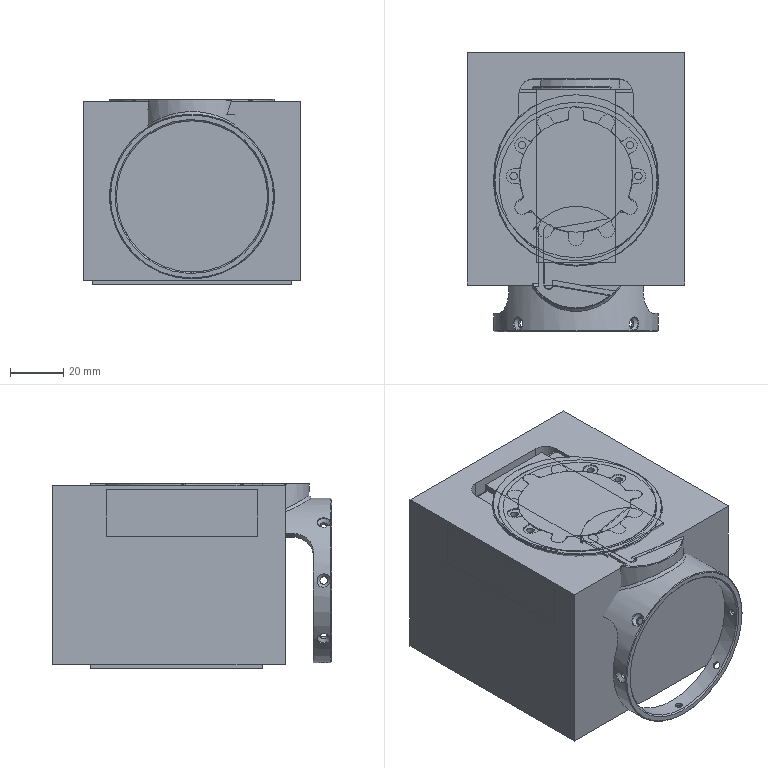NC program | NX | posted with a generic post | part box 82 x 105.2 x 70 mm
Whole program:
N10 G17 G21 G94 G90
(外形动态铣_1 , TOOL : 粗刀D16)
N12 T18 M6
N14 G53
N16 G17 G0 G90 X-3.784 Y5.106 B0. C0. S5500 M3
N18 G43 Z11. H18
N20 G94 G1 Z1. F3500.
N22 G3 X-3.784 Y5.106 Z-0.404 I3.765 J-5.175
N24 X-3.784 Y5.106 Z-1.808 I3.765 J-5.175
N26 X-3.784 Y5.106 Z-3.213 I3.765 J-5.175
N28 X-3.784 Y5.106 Z-4.617 I3.765 J-5.175
N30 X-3.784 Y5.106 Z-6.021 I3.765 J-5.175
N32 X-3.784 Y5.106 Z-7.425 I3.765 J-5.175
N34 X-3.784 Y5.106 Z-8.83 I3.765 J-5.175
N36 X-3.784 Y5.106 Z-10.234 I3.765 J-5.175
N38 X-3.784 Y5.106 Z-11.638 I3.765 J-5.175
N40 X-3.784 Y5.106 Z-13.042 I3.765 J-5.175
N42 X-3.784 Y5.106 Z-14.447 I3.765 J-5.175
N44 X-3.784 Y5.106 Z-15.851 I3.765 J-5.175
N46 X-3.784 Y5.106 Z-17.255 I3.765 J-5.175
N48 X-3.784 Y5.106 Z-18.659 I3.765 J-5.175
N50 X-3.784 Y5.106 Z-20.064 I3.765 J-5.175
N52 X-3.784 Y5.106 Z-21.468 I3.765 J-5.175
N54 X-3.784 Y5.106 Z-22.872 I3.765 J-5.175
N56 X-3.784 Y5.106 Z-24.276 I3.765 J-5.175
N58 X-3.784 Y5.106 Z-25.681 I3.765 J-5.175
N60 X-3.784 Y5.106 Z-27.085 I3.765 J-5.175
N62 X6.381 Y0.001 Z-28. R-6.4
N64 X-6.159 Y-1.924 R-6.417
N66 X5.583 Y-3.213 R6.447
N68 X4.619 Y5.05 R6.617
N70 X-2.015 Y6.615 R6.783
N72 X-1.429 Y-6.792 R6.922
N74 X5.428 Y-4.327 R6.966
N76 X5.458 Y4.871 R7.189
N78 X-1.347 Y7.296 R7.232
N80 X-3.143 Y-6.759 R7.43
N82 X5.315 Y-5.233 R7.495
N84 X6.334 Y4.554 R7.735
N86 X-1.413 Y7.816 R7.718
N88 X-3.194 Y-7.315 R7.955
N90 X5.195 Y-6.068 R8.031
N92 X7.227 Y4.092 R8.265
N94 X-0.67 Y8.452 R8.235
N96 X-7.198 Y-4.572 R8.485
N98 X4.491 Y-7.254 R8.542
N100 X7.344 Y4.986 R8.811
N102 X-2.79 Y8.608 R8.838
N104 X0.22 Y-9.083 R9.064
N106 X8.483 Y-3.519 R9.312
N108 X0.238 Y9.593 R9.335
N110 X-9.345 Y-2.455 R9.605
N112 X3.895 Y-8.848 R9.664
N114 X-0.068 Y10.184 R9.927
N116 X-10.127 Y-1.586 R10.185
N118 X3.436 Y-9.665 R10.249
N120 X0.291 Y10.777 R10.523
N122 X-10.229 Y-3.64 R10.794
N124 X3.073 Y-10.423 R10.868
N126 X0.292 Y11.389 R11.134
N128 X-11.409 Y-1.191 R11.396
N130 X3.05 Y-11.073 R11.48
N132 X0.983 Y11.971 R11.754
N134 X-12.028 Y1.278 R12.002
N136 X2.128 Y-11.927 R12.101
N138 X10.461 Y6.804 R12.376
N140 X-3.616 Y12.16 R12.464
N142 X-12.426 Y-2.837 R12.684
N144 X3.778 Y-12.193 R12.774
N146 X7.36 Y10.98 R13.028
N148 X-7.611 Y10.983 R13.201
N150 X-9.364 Y-9.587 R13.365
N152 X7.293 Y-11.291 R13.474
N154 X9.935 Y9.622 R13.683
N156 X-5.912 Y12.705 R13.82
N158 X-10.732 Y-9.093 R14.017
N160 X5.879 Y-12.813 R14.13
N162 X12.17 Y7.794 R14.342
N164 X-4.674 Y13.912 R14.454
N166 X-13.994 Y-4.617 R14.665
N168 X3.837 Y-14.256 R14.772
N170 X13.816 Y6.068 R15.006
N172 X-3.359 Y14.976 R15.109
N174 X-15.363 Y-1.292 R15.338
N176 X0.655 Y-15.424 R15.44
N178 X14.873 Y-4.712 R15.662
N180 X1.02 Y15.975 R15.77
N182 X-15.835 Y2.94 R15.998
N184 X-2.629 Y-15.909 R16.112
N186 X14.797 Y-6.767 R16.314
N188 X5.904 Y15.577 R16.449
N190 X-12.186 Y11.541 R16.613
N192 X-4.873 Y-16.102 R16.788
N194 X14.677 Y-8.494 R16.994
N196 X6.511 Y16.093 R17.151
N198 X-11.938 Y12.781 R17.303
N200 X-10.446 Y-14.08 R17.485
N202 X14.162 Y-10.535 R17.678
N204 X6.516 Y16.862 R17.862
N206 X-10.879 Y14.594 R18.008
N208 X-6.335 Y-17.116 R18.211
N210 X15.82 Y-9.382 R18.411
N212 X7.383 Y17.28 R18.587
N214 X-10.698 Y15.613 R18.722
N216 X-7.508 Y-17.431 R18.939
N218 X16.802 Y-9.147 R19.139
N220 X8.107 Y17.755 R19.32
N222 X-14.492 Y13.299 R19.465
N224 X-7.242 Y-18.336 R19.676
N226 X16.749 Y-10.661 R19.864
N228 X7.622 Y18.773 R20.055
N230 X-14.319 Y14.538 R20.185
N232 X-7.55 Y-19.009 R20.409
N234 X17.983 Y-10.066 R20.598
N236 X9.019 Y18.959 R20.799
N238 X-13.831 Y16.001 R20.934
N240 X-9.758 Y-18.822 R21.158
N242 X17.341 Y-12.438 R21.333
N244 X8.342 Y20.092 R21.557
N246 X-14.15 Y16.715 R21.672
N248 X-21.896 Y1.274 R21.879
N250 X-9.379 Y-19.854 R21.91
N252 X9.291 Y-19.973 R22.044
N254 X21.998 Y3.456 R22.247
N256 X5.042 Y21.975 R22.363
N258 X-12.269 Y19.039 R22.33
N260 X-22.588 Y2.165 R22.602
N262 X-18.471 Y-13.214 R22.645
N264 X4.912 Y-22.232 R22.818
N266 X10.783 Y-20.084 R23.104
N268 X16.696 Y15.519 R22.794
N270 G2 X15.722 Y16.62 R18.325
N272 G3 X12.958 Y19.176 R15.261
N274 X5.207 Y22.713 R21.966
N276 X-14.081 Y18.713 R23.157
N278 G1 X-14.407 Y18.466
N280 G3 X-14.7 Y18.163 R1.237
N282 G2 X-16.194 Y16.064 R10.91
N284 G3 X-18.085 Y13.88 R29.531
N286 X10.872 Y-20.036 R22.796
N288 X11.323 Y-19.376 R0.88
N290 G1 X11.502 Y-17.996
N292 X11.861 Y-15.219 Z-27.5
N294 X15.344 Y11.699 F15000.
N296 X15.704 Y14.476 Z-28. F3500.
N298 X15.897 Y15.97
N300 G3 X15.722 Y16.62 R0.88
N302 G2 X14.962 Y17.705 R13.92
N304 G3 X13.465 Y19.422 R8.461
N306 X9.979 Y21.752 R16.288
N308 X1.125 Y24.078 R22.494
N310 X-13.106 Y20.318 R23.892
N312 X-13.908 Y19.712 R6.441
N314 X-14.119 Y19.384 R1.156
N316 G2 X-14.721 Y18.126 R9.352
N318 G3 X-14.119 Y19.384 R9.352
N320 G1 X-14.029 Y19.617
N322 G2 X-13.258 Y20.558 R4.444
N324 X-11.121 Y22.12 R11.56
N326 X-6.152 Y24.122 R20.064
N328 X8.694 Y23.164 R23.732
N330 X13.001 Y20.706 R18.073
N332 X13.798 Y20.014 R10.677
N334 X14.001 Y19.687 R1.168
N336 G3 X14.962 Y17.705 R11.57
N338 G2 X14.001 Y19.687 R11.57
N340 G1 X13.933 Y19.864
N342 X13.928 Y19.878
N344 G3 X13.549 Y20.508 R2.958
N346 X11.795 Y22.164 R8.411
N348 X8.327 Y24.05 R16.01
N350 X0.534 Y25.637 R22.912
N352 X-8.61 Y24.13 R23.643
N354 X-11.988 Y22.402 R16.692
N356 X-13.452 Y21.178 R8.868
N358 X-13.647 Y20.823 R1.259
N360 G2 X-14.07 Y19.51 R9.633
N362 G3 X-13.647 Y20.823 R9.633
N364 G1 X-13.614 Y20.945
N366 X-13.608 Y20.97
N368 G2 X-13.432 Y21.357 R1.713
N370 X-12.263 Y22.691 R5.793
N372 X-9.129 Y24.615 R13.04
N374 X-3.244 Y26.219 R21.115
N376 X7.354 Y25.21 R23.909
N378 X11.351 Y23.303 R17.579
N380 X13.349 Y21.618 R9.929
N382 X13.553 Y21.23 R1.212
N384 G3 X13.928 Y19.878 R10.647
N386 G2 X13.553 Y21.23 R10.647
N388 G1 X13.527 Y21.353
N390 X13.496 Y21.474
N392 G3 X12.861 Y22.498 R4.095
N394 X11.022 Y24.122 R9.022
N396 X7.193 Y25.992 R15.979
N398 X-0.669 Y27.179 R23.165
N400 X-7.952 Y25.882 R22.825
N402 X-11.398 Y24.162 R15.64
N404 X-13.21 Y22.518 R8.421
N406 X-13.406 Y22.05 R1.101
N408 G2 X-13.608 Y20.97 R12.038
N410 G3 X-13.406 Y22.05 R12.038
N412 G1 X-13.377 Y22.302
N414 G2 X-12.763 Y23.399 R3.705
N416 X-11.222 Y24.846 R7.832
N418 X-7.996 Y26.564 R13.855
N420 X-3.514 Y27.704 R20.945
N422 X5.203 Y27.341 R23.775
N424 X9.416 Y25.86 R19.684
N426 X12.132 Y24.078 R12.486
N428 X13.222 Y22.868 R6.56
N430 X13.353 Y22.492 R1.266
N432 G3 X13.55 Y21.246 R10.987
N434 G2 X13.353 Y22.492 R10.987
N436 G1 X13.345 Y22.581
N438 X13.344 Y22.593
N440 X13.334 Y22.717
N442 G3 X12.779 Y23.815 R3.526
N444 X11.481 Y25.166 R7.411
N446 X8.291 Y27.063 R13.05
N448 X2.962 Y28.5 R20.694
N450 G1 X-2.038
N452 G3 X-8.998 Y26.91 R18.276
N454 X-11.775 Y25.212 R12.397
N456 X-13.142 Y23.717 R6.721
N458 X-13.31 Y23.214 R1.078
N460 G2 X-13.389 Y22.203 R8.714
N462 G3 X-13.31 Y23.214 R8.714
N464 G1 X-13.305 Y23.464
N466 G2 X-12.793 Y24.583 R3.38
N468 X-11.299 Y26.149 R7.293
N470 X-8.123 Y27.957 R12.789
N472 X-6.711 Y28.455 R16.875
N474 X-6.441 Y28.5 R1.43
N476 G1 X-1.941
N478 X-7.066
N480 G3 X-9.313 Y27.948 R7.391
N482 X-12.162 Y26.111 R9.158
N484 X-13.166 Y24.839 R5.937
N486 X-13.3 Y24.344 R1.098
N488 G1 Y23.678
N490 X-13.306 Y23.419
N492 X-13.3 Y23.669
N494 Y23.678
N496 Y24.594
N498 G2 X-12.833 Y25.744 R3.222
N500 X-10.942 Y27.638 R6.743
N502 X-9.454 Y28.442 R8.231
N504 X-9.164 Y28.5 R1.394
N506 G1 X-7.039
N508 X-9.414
N510 G3 X-10.929 Y28.029 R4.247
N512 X-13.19 Y25.899 R5.46
N514 X-13.3 Y25.489 R1.231
N516 G1 Y24.489
N518 Y25.614
N520 X-13.296 Y25.739
N522 G2 X-12.781 Y26.887 R3.143
N524 X-10.991 Y28.414 R4.876
N526 X-10.604 Y28.5 R1.271
N528 G1 X-9.354
N530 X-10.854
N532 G3 X-12.043 Y28.014 R3.036
N534 X-13.197 Y26.781 R3.655
N536 X-13.3 Y26.379 R1.245
N538 G1 Y25.504
N540 Y26.504
N542 X-13.297 Y26.629
N544 G2 X-12.908 Y27.489 R2.417
N546 X-11.914 Y28.39 R3.041
N548 X-11.504 Y28.5 R1.231
N550 G1 X-10.754
N552 X-11.629
N554 X-11.754 Y28.495
N556 G3 X-12.344 Y28.261 R2.142
N558 X-13.14 Y27.51 R2.729
N560 X-13.3 Y27.001 R1.076
N562 G1 Y26.501
N564 Y27.126
N566 X-13.295 Y27.251
N568 G2 X-13.042 Y27.816 R1.929
N570 X-12.501 Y28.351 R2.279
N572 X-12.038 Y28.5 R1.136
N574 G1 X-11.538
N576 X-12.163
N578 X-12.287 Y28.491
N580 X-12.587 Y28.374
N582 G3 X-13.043 Y28.03 R2.706
N584 X-13.3 Y27.428 R1.049
N586 G1 Y27.053
N588 Y27.593
N590 X-13.279 Y27.716
N592 G2 X-13.063 Y28.117 R3.623
N594 X-12.673 Y28.42 R0.885
N596 G1 X-12.407 Y28.5
N598 X-12.157
N600 X-12.407
N602 G3 X-13.3 Y27.593 R0.879
N604 G2 X-12.409 Y28.5 R0.879
N606 G1 X4.712
N608 G2 X8.039 Y27.822 R11.246
N610 X11.55 Y25.891 R12.34
N612 X13.006 Y24.351 R7.282
N614 X13.257 Y23.879 R1.791
N616 X13.301 Y23.617 R1.436
N618 G1 X13.312 Y23.138
N620 Y23.122
N622 X13.344 Y22.593
N624 X13.312 Y23.122
N626 Y23.138
N628 X13.301 Y23.617
N630 X13.3 Y23.678
N632 Y23.803
N634 X13.29 Y23.928
N636 G3 X12.777 Y25.075 R3.523
N638 X11.369 Y26.603 R6.912
N640 X8.026 Y28.459 R11.035
N642 X7.76 Y28.5 R1.433
N644 G1 X4.635
N646 X8.135
N648 G2 X9.709 Y28.125 R5.237
N650 X12.634 Y26.043 R7.414
N652 X13.21 Y25.181 R4.674
N654 X13.3 Y24.791 R1.265
N656 G1 Y23.791
N658 Y25.041
N660 G3 X12.984 Y25.924 R2.981
N662 X11.39 Y27.704 R5.681
N664 X10.183 Y28.416 R6.728
N666 X9.797 Y28.5 R1.272
N668 G1 X8.047
N670 X10.047
N672 G2 X11.239 Y28.127 R3.532
N674 X13.18 Y26.311 R4.781
N676 X13.3 Y25.89 R1.211
N678 G1 Y25.015
N680 Y26.015
N682 X13.294 Y26.139
N684 G3 X12.931 Y27.008 R2.792
N686 X11.404 Y28.408 R4.049
N688 X11.011 Y28.5 R1.262
N690 G1 X10.011
N692 X11.261
N694 G2 X12.385 Y27.984 R2.729
N696 X13.189 Y27.083 R3.134
N698 X13.3 Y26.673 R1.232
N700 G1 Y25.923
N702 Y26.798
N704 X13.294 Y26.923
N706 G3 X12.676 Y27.991 R2.365
N708 X12.255 Y28.345 R3.758
N710 X11.749 Y28.5 R1.08
N712 G1 X11.249
N714 X11.874
N716 X11.999 Y28.496
N718 G2 X12.592 Y28.229 R1.987
N720 X13.128 Y27.706 R2.438
N722 X13.3 Y27.158 R1.049
N724 G1 Y26.783
N726 Y27.283
N728 X13.297 Y27.408
N730 X13.198 Y27.704
N732 G3 X12.729 Y28.295 R1.98
N734 X12.203 Y28.5 R1.111
N736 G1 X11.828
N738 X12.328
N740 X12.453 Y28.486
N742 G2 X12.951 Y28.224 R2.134
N744 X13.235 Y27.82 R0.894
N746 G1 X13.3 Y27.58
N748 Y27.205
N750 Y27.58
N752 G3 X12.393 Y28.5 R0.88
N754 G1 X12.268
N756 G3 X11.568 Y28.095 R0.808
N758 G1 X9.781 Y24.996
N760 Z-27.
N762 G0 Z7.79
N764 X-3.784 Y5.106
N766 G1 Z-27.
N768 G3 X-3.784 Y5.106 Z-28.404 I3.765 J-5.175
N770 X-3.784 Y5.106 Z-29.808 I3.765 J-5.175
N772 X-3.784 Y5.106 Z-31.213 I3.765 J-5.175
N774 X-3.784 Y5.106 Z-32.617 I3.765 J-5.175
N776 X-3.784 Y5.106 Z-34.021 I3.765 J-5.175
N778 X-3.784 Y5.106 Z-35.425 I3.765 J-5.175
N780 X-3.784 Y5.106 Z-36.83 I3.765 J-5.175
N782 X-3.784 Y5.106 Z-38.234 I3.765 J-5.175
N784 X-3.784 Y5.106 Z-39.638 I3.765 J-5.175
N786 X-3.784 Y5.106 Z-41.042 I3.765 J-5.175
N788 X-3.784 Y5.106 Z-42.447 I3.765 J-5.175
N790 X-3.784 Y5.106 Z-43.851 I3.765 J-5.175
N792 X-3.784 Y5.106 Z-45.255 I3.765 J-5.175
N794 X-3.784 Y5.106 Z-46.659 I3.765 J-5.175
N796 X-3.784 Y5.106 Z-48.064 I3.765 J-5.175
N798 X-3.784 Y5.106 Z-49.468 I3.765 J-5.175
N800 X-3.784 Y5.106 Z-50.872 I3.765 J-5.175
N802 X-3.784 Y5.106 Z-52.276 I3.765 J-5.175
N804 X-3.784 Y5.106 Z-53.681 I3.765 J-5.175
N806 X-3.784 Y5.106 Z-55.085 I3.765 J-5.175
N808 X6.381 Y0.001 Z-56. R-6.4
N810 X-6.158 Y-1.924 R-6.417
N812 X5.584 Y-3.213 R6.447
N814 X4.619 Y5.05 R6.617
N816 X-2.331 Y6.512 R6.795
N818 X-0.273 Y-6.935 R6.924
N820 X5.428 Y-4.327 R6.977
N822 X5.459 Y4.871 R7.189
N824 X-1.347 Y7.297 R7.233
N826 X-2.827 Y-6.897 R7.431
N828 X5.315 Y-5.233 R7.499
N830 X6.431 Y4.406 R7.736
N832 X-0.707 Y7.908 R7.708
N834 X-3.194 Y-7.315 R7.955
N836 X5.195 Y-6.068 R8.024
N838 X7.05 Y4.411 R8.257
N840 X-0.854 Y8.437 R8.247
N842 X-6.887 Y-5.03 R8.49
N844 X5.103 Y-6.841 R8.547
N846 X7.24 Y5.143 R8.799
N848 X-2.789 Y8.608 R8.838
N850 X-0.161 Y-9.085 R9.063
N852 X7.534 Y-5.182 R9.286
N854 X0.238 Y9.593 R9.337
N856 X-9.346 Y-2.455 R9.605
N858 X4.075 Y-8.768 R9.667
N860 X4.76 Y8.933 R9.927
N862 X-7.324 Y7.14 R10.095
N864 X1.872 Y-10.083 R10.236
N866 X0.498 Y10.767 R10.522
N868 X-10.421 Y-3.047 R10.791
N870 X3.074 Y-10.424 R10.87
N872 X-0.136 Y11.395 R11.135
N874 X-11.458 Y-0.551 R11.396
N876 X2.843 Y-11.128 R11.479
N878 X1.419 Y11.922 R11.754
N880 X-11.939 Y1.931 R11.996
N882 X1.693 Y-11.996 R12.098
N884 X10.689 Y6.419 R12.372
N886 X-2.522 Y12.425 R12.447
N888 X-12.518 Y-2.395 R12.677
N890 X3.56 Y-12.257 R12.768
N892 X5.982 Y11.811 R13.028
N894 X-10.619 Y8.133 R13.226
N896 X-0.184 Y-13.406 R13.385
N898 X13.639 Y0.244 R13.639
N900 X-0.416 Y13.967 R13.736
N902 X-14.044 Y-0.64 R13.972
N904 X2.25 Y-13.899 R14.075
N906 X12.967 Y6.311 R14.329
N908 X-3.977 Y14.12 R14.436
N910 X-14.139 Y-4.154 R14.659
N912 X2.411 Y-14.559 R14.764
N914 X14.879 Y2.044 R14.99
N916 X-1.153 Y15.289 R15.093
N918 X-15.387 Y0.94 R15.328
N920 X0.158 Y-15.435 R15.434
N922 X14.95 Y-4.475 R15.656
N924 X0.769 Y15.991 R15.77
N926 X-16.018 Y1.685 R16.003
N928 X-2.378 Y-15.949 R16.115
N930 X14.797 Y-6.767 R16.316
N932 X5.904 Y15.576 R16.449
N934 X-12.185 Y11.541 R16.612
N936 X-4.873 Y-16.102 R16.788
N938 X14.677 Y-8.495 R16.995
N940 X7.235 Y15.771 R17.152
N942 X-11.343 Y13.308 R17.291
N944 X-12.814 Y-11.966 R17.481
N946 X11.417 Y-13.415 R17.652
N948 X8.698 Y15.816 R17.852
N950 X-10.877 Y14.594 R17.993
N952 X-6.337 Y-17.115 R18.209
N954 X15.819 Y-9.385 R18.411
N956 X7.636 Y17.167 R18.588
N958 X-10.922 Y15.457 R18.716
N960 X-6.228 Y-17.929 R18.939
N962 X16.934 Y-8.907 R19.145
N964 X8.111 Y17.754 R19.325
N966 X-13.503 Y14.298 R19.457
N968 X-5.923 Y-18.804 R19.675
N970 X15.052 Y-12.914 R19.857
N972 X7.889 Y18.66 R20.054
N974 X-14.109 Y14.739 R20.178
N976 X-7.555 Y-19.008 R20.409
N978 X18.26 Y-9.569 R20.604
N980 X7.968 Y19.436 R20.805
N982 X-13.826 Y16.005 R20.934
N984 X-10.02 Y-18.684 R21.161
N986 X18.613 Y-10.482 R21.347
N988 X8.887 Y19.851 R21.56
N990 X-14.593 Y16.332 R21.675
N992 X-21.894 Y1.279 R21.881
N994 X-8.575 Y-20.219 R21.921
N996 X18.614 Y-11.93 R22.097
N998 X5.92 Y21.742 R22.321
N1000 X-13.014 Y18.542 R22.361
N1002 X-22.613 Y1.871 R22.609
N1004 X-5.848 Y-21.962 R22.703
N1006 X5.2 Y-22.167 R22.71
N1008 X10.715 Y-20.12 R23.004
N1010 X16.69 Y15.526 R22.795
N1012 G2 X15.721 Y16.62 R18.188
N1014 G3 X12.956 Y19.179 R15.281
N1016 X5.492 Y22.642 R21.912
N1018 X-14.078 Y18.714 R23.143
N1020 G1 X-14.406 Y18.466
N1022 G3 X-14.7 Y18.162 R1.234
N1024 G2 X-16.194 Y16.064 R10.909
N1026 G3 X-18.072 Y13.896 R29.639
N1028 X10.748 Y-20.103 R22.796
N1030 X11.199 Y-19.446 R0.88
N1032 G1 X11.379 Y-18.085
N1034 X11.748 Y-15.309 Z-55.5
N1036 X15.332 Y11.715 F15000.
N1038 X15.7 Y14.49 Z-56. F3500.
N1040 X15.896 Y15.967
N1042 G3 X15.721 Y16.62 R0.88
N1044 G2 X14.961 Y17.705 R13.94
N1046 G3 X13.466 Y19.423 R8.452
N1048 X9.98 Y21.751 R16.271
N1050 X1.125 Y24.078 R22.52
N1052 X-13.106 Y20.318 R23.897
N1054 X-13.908 Y19.711 R6.45
N1056 X-14.119 Y19.384 R1.156
N1058 G2 X-14.72 Y18.126 R9.365
N1060 G3 X-14.119 Y19.384 R9.365
N1062 G1 X-14.029 Y19.617
N1064 G2 X-13.258 Y20.558 R4.446
N1066 X-11.121 Y22.12 R11.558
N1068 X-6.152 Y24.121 R20.055
N1070 X8.694 Y23.164 R23.737
N1072 X13.001 Y20.707 R18.061
N1074 X13.798 Y20.015 R10.649
N1076 X14.001 Y19.688 R1.168
N1078 G3 X14.961 Y17.705 R11.57
N1080 G2 X14.001 Y19.688 R11.57
N1082 G1 X13.933 Y19.864
N1084 X13.927 Y19.879
N1086 G3 X13.55 Y20.508 R2.889
N1088 X11.795 Y22.164 R8.406
N1090 X8.327 Y24.05 R16.011
N1092 X0.534 Y25.637 R22.915
N1094 X-8.61 Y24.13 R23.649
N1096 X-11.988 Y22.402 R16.688
N1098 X-13.452 Y21.178 R8.87
N1100 X-13.647 Y20.822 R1.257
N1102 G2 X-14.07 Y19.51 R9.664
N1104 G3 X-13.647 Y20.822 R9.664
N1106 G1 X-13.614 Y20.945
N1108 X-13.608 Y20.97
N1110 G2 X-13.432 Y21.357 R1.711
N1112 X-12.263 Y22.691 R5.793
N1114 X-9.129 Y24.614 R13.039
N1116 X-3.244 Y26.219 R21.12
N1118 X7.354 Y25.209 R23.909
N1120 X11.352 Y23.303 R17.579
N1122 X13.351 Y21.611 R10.127
N1124 X13.554 Y21.225 R1.214
N1126 G3 X13.927 Y19.879 R10.762
N1128 G2 X13.554 Y21.225 R10.762
N1130 G1 X13.528 Y21.347
N1132 X13.497 Y21.468
N1134 G3 X12.819 Y22.545 R4.126
N1136 X11.283 Y23.938 R8.758
N1138 X7.735 Y25.797 R15.229
N1140 X0.535 Y27.171 R22.583
N1142 X-7.348 Y26.089 R23.438
N1144 X-11.397 Y24.162 R16.154
N1146 X-13.21 Y22.521 R8.295
N1148 X-13.406 Y22.054 R1.099
N1150 G2 X-13.608 Y20.97 R12.037
N1152 G3 X-13.406 Y22.054 R12.037
N1154 G1 X-13.377 Y22.302
N1156 G2 X-12.802 Y23.352 R3.473
N1158 X-11.222 Y24.845 R7.877
N1160 X-7.996 Y26.564 R13.858
N1162 X-3.514 Y27.704 R20.948
N1164 X5.202 Y27.341 R23.775
N1166 X9.416 Y25.86 R19.682
N1168 X12.131 Y24.078 R12.463
N1170 X13.221 Y22.868 R6.592
N1172 X13.353 Y22.491 R1.264
N1174 G3 X13.549 Y21.246 R10.942
N1176 G2 X13.353 Y22.491 R10.942
N1178 G1 X13.345 Y22.581
N1180 X13.344 Y22.593
N1182 X13.333 Y22.717
N1184 G3 X12.778 Y23.815 R3.528
N1186 X11.481 Y25.166 R7.406
N1188 X8.29 Y27.063 R13.046
N1190 X2.961 Y28.5 R20.691
N1192 G1 X-2.039
N1194 G3 X-8.998 Y26.91 R18.28
N1196 X-11.777 Y25.211 R12.345
N1198 X-13.141 Y23.72 R6.667
N1200 X-13.31 Y23.216 R1.078
N1202 G2 X-13.388 Y22.203 R8.716
N1204 G3 X-13.31 Y23.216 R8.716
N1206 G1 X-13.305 Y23.466
N1208 G2 X-12.795 Y24.582 R3.366
N1210 X-11.299 Y26.149 R7.296
N1212 X-8.123 Y27.957 R12.793
N1214 X-6.711 Y28.455 R16.879
N1216 X-6.442 Y28.5 R1.427
N1218 G1 X-1.942
N1220 X-7.067
N1222 G3 X-9.314 Y27.948 R7.393
N1224 X-12.164 Y26.111 R9.16
N1226 X-13.192 Y24.788 R5.783
N1228 X-13.3 Y24.381 R1.237
N1230 G1 Y23.678
N1232 Y23.668
N1234 X-13.306 Y23.419
N1236 X-13.3 Y23.668
N1238 Y23.678
N1240 Y24.506
N1242 X-13.297 Y24.631
N1244 G2 X-12.799 Y25.796 R3.369
N1246 X-10.943 Y27.638 R6.756
N1248 X-9.454 Y28.442 R8.237
N1250 X-9.165 Y28.5 R1.393
N1252 G1 X-7.04
N1254 X-9.415
N1256 G3 X-10.931 Y28.029 R4.279
N1258 X-13.131 Y26.001 R5.517
N1260 X-13.3 Y25.486 R1.121
N1262 G1 Y24.486
N1264 Y25.611
N1266 X-13.296 Y25.736
N1268 G2 X-12.78 Y26.888 R3.147
N1270 X-10.991 Y28.414 R4.871
N1272 X-10.604 Y28.5 R1.271
N1274 G1 X-9.354
N1276 X-10.854
N1278 G3 X-12.043 Y28.014 R3.034
N1280 X-13.158 Y26.85 R3.732
N1282 X-13.3 Y26.352 R1.09
N1284 G1 Y25.602
N1286 Y26.602
N1288 G2 X-12.927 Y27.46 R2.364
N1290 X-11.949 Y28.373 R3.144
N1292 X-11.456 Y28.5 R1.107
N1294 G1 X-10.831
N1296 X-11.706
N1298 G3 X-12.571 Y28.107 R2.184
N1300 X-13.17 Y27.465 R2.762
N1302 X-13.3 Y26.972 R1.103
N1304 G1 Y26.597
N1306 Y27.222
N1308 X-13.282 Y27.345
N1310 G2 X-12.754 Y28.153 R2.067
N1312 X-12.013 Y28.5 R1.034
N1314 G1 X-11.638
N1316 X-12.138
N1318 X-12.263 Y28.496
N1320 X-12.56 Y28.387
N1322 G3 X-13.028 Y28.053 R2.734
N1324 X-13.3 Y27.443 R1.074
N1326 G1 Y27.193
N1328 Y27.593
N1330 G2 X-13.246 Y27.837 R1.183
N1332 X-12.988 Y28.209 R2.61
N1334 X-12.679 Y28.418 R0.891
N1336 G1 X-12.41 Y28.5
N1338 X-12.034
N1340 X-12.409
N1342 G3 X-13.3 Y27.593 R0.879
N1344 G2 X-12.409 Y28.5 R0.879
N1346 G1 X4.711
N1348 G2 X8.039 Y27.822 R11.245
N1350 X11.549 Y25.891 R12.336
N1352 X13.005 Y24.351 R7.283
N1354 X13.257 Y23.879 R1.808
N1356 X13.301 Y23.617 R1.435
N1358 G1 X13.312 Y23.138
N1360 Y23.122
N1362 X13.344 Y22.593
N1364 X13.312 Y23.122
N1366 Y23.138
N1368 X13.301 Y23.617
N1370 X13.3 Y23.678
N1372 Y23.803
N1374 G3 X13.206 Y24.228 R1.694
N1376 X12.242 Y25.767 R4.851
N1378 X10.038 Y27.528 R9.164
N1380 X8.026 Y28.458 R11.18
N1382 X7.76 Y28.5 R1.432
N1384 G1 X4.635
N1386 X8.135
N1388 G2 X9.709 Y28.125 R5.237
N1390 X12.634 Y26.042 R7.413
N1392 X13.21 Y25.18 R4.672
N1394 X13.3 Y24.789 R1.265
N1396 G1 Y23.789
N1398 Y25.039
N1400 G3 X12.984 Y25.923 R2.984
N1402 X11.39 Y27.704 R5.681
N1404 X10.183 Y28.416 R6.728
N1406 X9.797 Y28.5 R1.273
N1408 G1 X8.047
N1410 X10.047
N1412 G2 X11.239 Y28.127 R3.532
N1414 X13.18 Y26.31 R4.781
N1416 X13.3 Y25.819 R1.117
N1418 G1 Y24.944
N1420 Y26.069
N1422 G3 X12.815 Y27.179 R2.768
N1424 X11.421 Y28.393 R3.99
N1426 X11.015 Y28.5 R1.239
N1428 G1 X10.015
N1430 X11.14
N1432 X11.265 Y28.497
N1434 G2 X12.396 Y27.972 R2.715
N1436 X13.171 Y27.118 R3.31
N1438 X13.3 Y26.625 R1.104
N1440 G1 Y26.
N1442 Y26.875
N1444 G3 X13.074 Y27.468 R2.097
N1446 X12.278 Y28.326 R2.908
N1448 X11.76 Y28.5 R1.126
N1450 G1 X11.135
N1452 X11.885
N1454 X12.01 Y28.494
N1456 G2 X12.592 Y28.23 R1.997
N1458 X13.141 Y27.682 R2.46
N1460 X13.3 Y27.193 R1.097
N1462 G1 Y26.818
N1464 Y27.318
N1466 X13.291 Y27.443
N1468 X13.179 Y27.742
N1470 G3 X12.667 Y28.332 R1.925
N1472 X12.17 Y28.5 R1.089
N1474 G1 X11.795
N1476 X12.295
N1478 X12.42 Y28.49
N1480 G2 X12.937 Y28.232 R2.172
N1482 X13.229 Y27.834 R0.89
N1484 G1 X13.3 Y27.582
N1486 Y27.207
N1488 Y27.582
N1490 G3 X12.393 Y28.5 R0.88
N1492 G1 X12.268
N1494 G3 X11.568 Y28.095 R0.808
N1496 G1 X9.781 Y24.996
N1498 Z-55.
N1500 G0 Z11.
N1502 X-1.714 Y6.103
N1504 G1 Z-55.
N1506 G3 X-1.714 Y6.103 Z-56.404 I1.694 J-6.172
N1508 X6.38 Y0.001 Z-57.4 R-6.4
N1510 X-6.159 Y-1.924 R-6.417
N1512 X5.583 Y-3.213 R6.447
N1514 X4.618 Y5.05 R6.617
N1516 X-2.642 Y6.394 R6.795
N1518 X2.187 Y-6.581 R6.926
N1520 X5.533 Y-4.197 R7.075
N1522 X5.458 Y4.871 R7.187
N1524 X-1.178 Y7.324 R7.224
N1526 X-1.167 Y-7.36 R7.432
N1528 X5.435 Y-5.108 R7.52
N1530 X6.233 Y4.702 R7.729
N1532 X-1.764 Y7.745 R7.719
N1534 X-2.012 Y-7.725 R7.957
N1536 X5.058 Y-6.179 R8.035
N1538 X7.047 Y4.414 R8.264
N1540 X-0.857 Y8.435 R8.232
N1542 X-6.885 Y-5.034 R8.49
N1544 X5.255 Y-6.728 R8.552
N1546 X7.339 Y4.99 R8.808
N1548 X-2.062 Y8.804 R8.82
N1550 X-2.413 Y-8.763 R9.06
N1552 X7.188 Y-5.631 R9.223
N1554 X-0.358 Y9.595 R9.338
N1556 X-8.568 Y-4.476 R9.618
N1558 X4.083 Y-8.765 R9.68
N1560 X-0.683 Y10.166 R9.929
N1562 X-9.394 Y-4.114 R10.201
N1564 X3.824 Y-9.522 R10.263
N1566 X0.074 Y10.782 R10.525
N1568 X-10.577 Y-2.451 R10.791
N1570 X3.28 Y-10.36 R10.862
N1572 X0.495 Y11.38 R11.134
N1574 X-11.47 Y-0.132 R11.393
N1576 X2.223 Y-11.266 R11.472
N1578 X1.409 Y11.924 R11.752
N1580 X-11.941 Y1.922 R12.001
N1582 X1.482 Y-12.022 R12.095
N1584 X8.954 Y8.759 R12.377
N1586 X-4.901 Y11.711 R12.491
N1588 X-10.286 Y-7.536 R12.7
N1590 X3.998 Y-12.121 R12.768
N1592 X7.352 Y10.985 R13.03
N1594 X-9.064 Y9.827 R13.202
N1596 X0.054 Y-13.41 R13.382
N1598 X12.589 Y5.502 R13.657
N1600 X-1.84 Y13.864 R13.749
N1602 X-13.994 Y-1.357 R13.98
N1604 X2.02 Y-13.934 R14.065
N1606 X12.287 Y7.593 R14.334
N1608 X-3.987 Y14.119 R14.438
N1610 X-14.653 Y-1.548 R14.658
N1612 X2.417 Y-14.558 R14.747
N1614 X12.807 Y8.047 R15.012
N1616 X-3.368 Y14.974 R15.115
N1618 X-15.016 Y-3.506 R15.343
N1620 X2.146 Y-15.293 R15.433
N1622 X13.801 Y7.692 R15.697
N1624 X-3.024 Y15.749 R15.806
N1626 X-15.895 Y-2.625 R16.029
N1628 X2.691 Y-15.913 R16.129
N1630 X15.258 Y6.189 R16.382
N1632 X-4.515 Y16.127 R16.507
N1634 X-15.178 Y-7.244 R16.75
N1636 X4.362 Y-16.276 R16.863
N1638 X15.077 Y8.283 R17.098
N1640 X-8.994 Y14.986 R17.244
N1642 X-7.247 Y-15.968 R17.492
N1644 X15.861 Y-7.819 R17.709
N1646 X5.23 Y17.318 R17.879
N1648 X-11.74 Y13.911 R18.011
N1650 X-5.808 Y-17.305 R18.213
N1652 X16.489 Y-8.178 R18.425
N1654 X6.086 Y17.795 R18.601
N1656 X-13.654 Y13.117 R18.738
N1658 X-4.886 Y-18.345 R18.944
N1660 X17.669 Y-7.386 R19.164
N1662 X5.739 Y18.682 R19.34
N1664 X-14.883 Y12.857 R19.467
N1666 X-6.952 Y-18.45 R19.674
N1668 X17.625 Y-9.177 R19.884
N1670 X6.258 Y19.288 R20.075
N1672 X-15.698 Y13.043 R20.209
N1674 X-10.093 Y-17.791 R20.416
N1676 X16.236 Y-12.649 R20.596
N1678 X8.983 Y18.978 R20.806
N1680 X-17.019 Y12.57 R20.958
N1682 X-9.2 Y-19.103 R21.163
N1684 X19.797 Y-8.077 R21.361
N1686 X5.796 Y20.993 R21.563
N1688 X-17.263 Y13.496 R21.704
N1690 X-12.659 Y-17.936 R21.917
N1692 X18.312 Y-12.377 R22.094
N1694 X11.364 Y19.399 R22.312
N1696 X-15.624 Y16.416 R22.444
N1698 X-11.345 Y-19.681 R22.675
N1700 X4.964 Y-22.215 R22.811
N1702 X10.694 Y-20.127 R23.031
N1704 X16.686 Y15.522 R22.79
N1706 G2 X15.724 Y16.609 R18.201
N1708 G3 X12.773 Y19.305 R14.977
N1710 X4.73 Y22.818 R21.83
N1712 X-14.503 Y18.387 R23.152
N1714 X-14.694 Y18.164 R1.398
N1716 G2 X-16.186 Y16.066 R10.951
N1718 G3 X-18.068 Y13.892 R29.712
N1720 X10.744 Y-20.099 R22.791
N1722 X11.196 Y-19.442 R0.88
N1724 G1 X11.377 Y-18.08
N1726 X11.745 Y-15.304 Z-56.9
N1728 X15.334 Y11.704 F15000.
N1730 X15.702 Y14.48 Z-57.4 F3500.
N1732 X15.899 Y15.956
N1734 G3 X15.724 Y16.609 R0.88
N1736 G2 X14.899 Y17.804 R11.892
N1738 G3 X13.35 Y19.525 R8.77
N1740 X9.887 Y21.798 R16.512
N1742 X1.616 Y24.039 R22.5
N1744 X-13.106 Y20.318 R23.852
N1746 X-13.904 Y19.713 R6.326
N1748 X-14.113 Y19.386 R1.157
N1750 G2 X-14.713 Y18.13 R9.317
N1752 G3 X-14.113 Y19.386 R9.317
N1754 G1 X-14.023 Y19.619
N1756 G2 X-13.212 Y20.598 R4.419
N1758 X-10.853 Y22.274 R12.032
N1760 X-5.295 Y24.325 R20.67
N1762 X8.496 Y23.243 R23.813
N1764 X12.897 Y20.788 R18.379
N1766 X13.816 Y19.992 R8.898
N1768 X13.974 Y19.743 R1.394
N1770 G3 X14.961 Y17.696 R11.702
N1772 G2 X13.974 Y19.743 R11.702
N1774 G1 X13.925 Y19.869
N1776 G3 X13.72 Y20.259 R2.087
N1778 X12.475 Y21.627 R6.725
N1780 X9.301 Y23.623 R14.197
N1782 X2.811 Y25.454 R21.75
N1784 X-8.107 Y24.317 R24.005
N1786 X-11.726 Y22.575 R17.632
N1788 X-13.448 Y21.178 R9.133
N1790 X-13.642 Y20.823 R1.26
N1792 G2 X-14.061 Y19.52 R9.605
N1794 G3 X-13.642 Y20.823 R9.605
N1796 G1 X-13.606 Y20.956
N1798 X-13.57 Y21.076
N1800 G2 X-12.881 Y22.083 R3.983
N1802 X-11.307 Y23.414 R8.844
N1804 X-7.778 Y25.152 R15.566
N1806 X-0.17 Y26.411 R22.984
N1808 X7.753 Y25.068 R23.54
N1810 X11.562 Y23.162 R17.094
N1812 X13.347 Y21.617 R9.736
N1814 X13.547 Y21.232 R1.217
N1816 G3 X13.925 Y19.869 R10.471
N1818 G2 X13.547 Y21.232 R10.471
N1820 G1 X13.522 Y21.354
N1822 X13.491 Y21.475
N1824 G3 X12.815 Y22.548 R4.084
N1826 X11.288 Y23.933 R8.767
N1828 X7.823 Y25.762 R15.076
N1830 X0.929 Y27.152 R22.473
N1832 X-7.259 Y26.116 R23.512
N1834 X-11.206 Y24.286 R16.311
N1836 X-12.949 Y22.824 R8.906
N1838 X-13.273 Y22.416 R3.156
N1840 X-13.401 Y22.051 R1.157
N1842 G1 X-13.402 Y22.043
N1844 X-13.491 Y21.5
N1846 X-13.606 Y20.956
N1848 X-13.491 Y21.5
N1850 X-13.402 Y22.043
N1852 X-13.372 Y22.299
N1854 G2 X-12.799 Y23.349 R3.461
N1856 X-11.223 Y24.842 R7.861
N1858 X-7.816 Y26.63 R14.114
N1860 X-3.325 Y27.727 R21.182
N1862 X6.311 Y27.052 R23.578
N1864 X10.589 Y25.21 R17.284
N1866 X12.668 Y23.556 R10.067
N1868 X13.228 Y22.855 R4.945
N1870 X13.348 Y22.486 R1.155
N1872 G1 X13.402 Y22.043
N1874 X13.491 Y21.5
N1876 X13.543 Y21.255
N1878 X13.491 Y21.5
N1880 X13.402 Y22.043
N1882 X13.348 Y22.49
N1884 X13.34 Y22.584
N1886 X13.332 Y22.708
N1888 G3 X12.923 Y23.598 R3.181
N1890 X11.663 Y25.009 R6.66
N1892 X8.792 Y26.837 R12.508
N1894 X3.578 Y28.404 R19.811
N1896 G1 X2.974 Y28.495
N1898 X-2.026
N1900 G3 X-9.001 Y26.906 R18.217
N1902 X-11.779 Y25.204 R12.312
N1904 X-13.137 Y23.718 R6.652
N1906 X-13.305 Y23.215 R1.078
N1908 G1 X-13.307 Y23.13
N1910 X-13.339 Y22.586
N1912 X-13.382 Y22.214
N1914 X-13.339 Y22.586
N1916 X-13.307 Y23.13
N1918 X-13.3 Y23.465
N1920 G2 X-12.793 Y24.578 R3.352
N1922 X-11.3 Y26.145 R7.283
N1924 X-8.126 Y27.953 R12.77
N1926 X-6.716 Y28.451 R16.83
N1928 X-6.447 Y28.495 R1.429
N1930 G1 X-1.947
N1932 X-7.072
N1934 G3 X-9.317 Y27.943 R7.377
N1936 X-12.161 Y26.108 R9.146
N1938 X-13.17 Y24.824 R5.822
N1940 X-13.295 Y24.332 R1.109
N1942 G1 Y23.676
N1944 X-13.3 Y23.426
N1946 X-13.295 Y23.676
N1948 Y24.582
N1950 G2 X-13.192 Y25.016 R1.855
N1952 X-12.395 Y26.337 R4.56
N1954 X-9.505 Y28.417 R7.848
N1956 X-9.123 Y28.495 R1.155
N1958 G1 X-6.998
N1960 X-9.373
N1962 G3 X-10.582 Y28.185 R3.862
N1964 X-13.148 Y25.975 R5.564
N1966 X-13.295 Y25.474 R1.087
N1968 G1 Y24.474
N1970 Y25.724
N1972 G2 X-12.952 Y26.612 R2.901
N1974 X-10.998 Y28.406 R4.788
N1976 X-10.608 Y28.495 R1.267
N1978 G1 X-9.358
N1980 X-10.858
N1982 G3 X-12.043 Y28.01 R3.021
N1984 X-13.181 Y26.809 R3.669
N1986 X-13.295 Y26.394 R1.224
N1988 G1 Y25.644
N1990 Y26.519
N1992 X-13.289 Y26.644
N1994 G2 X-12.908 Y27.484 R2.456
N1996 X-11.915 Y28.385 R3.038
N1998 X-11.505 Y28.495 R1.231
N2000 G1 X-10.755
N2002 X-11.63
N2004 X-11.754 Y28.49
N2006 G3 X-12.344 Y28.256 R2.15
N2008 X-13.13 Y27.519 R2.737
N2010 X-13.295 Y27.008 R1.118
N2012 G1 Y26.508
N2014 Y27.133
N2016 X-13.289 Y27.258
N2018 G2 X-13.042 Y27.81 R1.886
N2020 X-12.5 Y28.346 R2.279
N2022 X-12.037 Y28.495 R1.136
N2024 G1 X-11.537
N2026 X-12.162
N2028 X-12.287 Y28.486
N2030 X-12.586 Y28.369
N2032 G3 X-13.042 Y28.026 R2.705
N2034 X-13.295 Y27.425 R1.043
N2036 G1 Y27.05
N2038 Y27.588
N2040 G2 X-13.241 Y27.832 R1.164
N2042 X-12.995 Y28.196 R2.579
N2044 X-12.69 Y28.409 R0.888
N2046 G1 X-12.415 Y28.495
N2048 X-12.404
N2050 X-12.154
N2052 X-12.404
N2054 X-12.415
N2056 G3 X-13.295 Y27.588 R0.878
N2058 G2 X-12.404 Y28.495 R0.879
N2060 G1 X4.724
N2062 G2 X8.034 Y27.821 R11.181
N2064 X11.546 Y25.891 R12.34
N2066 X13.003 Y24.35 R7.174
N2068 X13.253 Y23.876 R1.764
N2070 X13.296 Y23.616 R1.439
N2072 G1 X13.307 Y23.13
N2074 X13.337 Y22.631
N2076 X13.307 Y23.13
N2078 X13.295 Y23.671
N2080 Y23.796
N2082 X13.286 Y23.92
N2084 G3 X12.773 Y25.073 R3.525
N2086 X11.364 Y26.602 R6.887
N2088 X8.023 Y28.456 R10.977
N2090 X7.759 Y28.495 R1.437
N2092 G1 X4.634
N2094 X8.134
N2096 G2 X9.928 Y28.032 R5.542
N2098 X12.744 Y25.899 R7.267
N2100 X13.199 Y25.204 R5.259
N2102 X13.295 Y24.808 R1.256
N2104 G1 Y23.683
N2106 Y25.058
N2108 G3 X12.972 Y25.939 R2.906
N2110 X11.384 Y27.7 R5.64
N2112 X10.178 Y28.412 R6.653
N2114 X9.793 Y28.495 R1.273
N2116 G1 X8.043
N2118 X10.043
N2120 G2 X11.233 Y28.123 R3.539
N2122 X13.175 Y26.311 R4.775
N2124 X13.295 Y25.82 R1.116
N2126 G1 Y24.945
N2128 Y26.07
N2130 G3 X12.812 Y27.175 R2.749
N2132 X11.418 Y28.388 R3.992
N2134 X11.012 Y28.495 R1.238
N2136 G1 X10.012
N2138 X11.137
N2140 X11.262 Y28.492
N2142 G2 X12.393 Y27.968 R2.716
N2144 X13.168 Y27.114 R3.294
N2146 X13.295 Y26.621 R1.106
N2148 G1 Y25.996
N2150 Y26.871
N2152 G3 X13.069 Y27.466 R2.097
N2154 X12.275 Y28.321 R2.903
N2156 X11.757 Y28.495 R1.126
N2158 G1 X11.132
N2160 X11.882
N2162 X12.006 Y28.489
N2164 G2 X12.588 Y28.225 R1.994
N2166 X13.136 Y27.678 R2.454
N2168 X13.295 Y27.189 R1.096
N2170 G1 Y26.814
N2172 Y27.314
N2174 X13.287 Y27.438
N2176 X13.174 Y27.738
N2178 G3 X12.663 Y28.328 R1.922
N2180 X12.166 Y28.495 R1.089
N2182 G1 X11.791
N2184 X12.291
N2186 X12.416 Y28.485
N2188 G2 X12.933 Y28.227 R2.17
N2190 X13.225 Y27.829 R0.89
N2192 G1 X13.295 Y27.578
N2194 Y27.203
N2196 Y27.578
N2198 G3 X12.388 Y28.495 R0.88
N2200 G1 X12.263
N2202 G3 X11.563 Y28.09 R0.808
N2204 G1 X9.777 Y24.991
N2206 Z-56.4
N2208 G0 Z11.
N2210 M5
(单向轮廓精光_6 , TOOL : T型刀D20-8)
N2212 T17 M6
N2214 G53
N2216 G17 G0 G90 X14.967 Y-1. B0. C0. S1500 M3
N2218 G43 Z11. H17
N2220 Z-20.211
N2222 G94 G1 Z-23.211 F800.
N2224 G41 X20.2 D17
N2226 G3 X21.2 Y0. R1.
N2228 X0. Y21.2 R21.2
N2230 X21.2 Y0. R-21.2
N2232 X21.194 Y0.5 R21.2
N2234 X20.171 Y1.476 R1.
N2236 G40
N2238 G1 X19.971 Y1.471
N2240 X20.1 Y-1.
N2242 G41 X20.3
N2244 G3 X21.3 Y0. R1.
N2246 X0. Y21.3 R21.3
N2248 X21.3 Y0. R-21.3
N2250 X21.294 Y0.5 R21.3
N2252 X20.271 Y1.476 R1.
N2254 G1 X15.24 Y1.358
N2256 G40
N2258 X15.04 Y1.353
N2260 Z-20.211
N2262 G0 Z11.
N2264 X14.967 Y-1.
N2266 Z-25.923
N2268 G1 Z-28.923
N2270 G41 X20.2
N2272 G3 X21.2 Y0. R1.
N2274 X0. Y21.2 R21.2
N2276 X21.2 Y0. R-21.2
N2278 X21.194 Y0.5 R21.2
N2280 X20.171 Y1.476 R1.
N2282 G40
N2284 G1 X19.971 Y1.471
N2286 X20.1 Y-1.
N2288 G41 X20.3
N2290 G3 X21.3 Y0. R1.
N2292 X0. Y21.3 R21.3
N2294 X21.3 Y0. R-21.3
N2296 X21.294 Y0.5 R21.3
N2298 X20.271 Y1.476 R1.
N2300 G1 X15.24 Y1.358
N2302 G40
N2304 X15.04 Y1.353
N2306 Z-25.923
N2308 G0 Z11.
N2310 X14.967 Y-1.
N2312 Z-31.634
N2314 G1 Z-34.634
N2316 G41 X20.2
N2318 G3 X21.2 Y0. R1.
N2320 X0. Y21.2 R21.2
N2322 X21.2 Y0. R-21.2
N2324 X21.194 Y0.5 R21.2
N2326 X20.171 Y1.476 R1.
N2328 G40
N2330 G1 X19.971 Y1.471
N2332 X20.1 Y-1.
N2334 G41 X20.3
N2336 G3 X21.3 Y0. R1.
N2338 X0. Y21.3 R21.3
N2340 X21.3 Y0. R-21.3
N2342 X21.294 Y0.5 R21.3
N2344 X20.271 Y1.476 R1.
N2346 G1 X15.24 Y1.358
N2348 G40
N2350 X15.04 Y1.353
N2352 Z-31.634
N2354 G0 Z11.
N2356 X14.967 Y-1.
N2358 Z-37.346
N2360 G1 Z-40.346
N2362 G41 X20.2
N2364 G3 X21.2 Y0. R1.
N2366 X0. Y21.2 R21.2
N2368 X21.2 Y0. R-21.2
N2370 X21.194 Y0.5 R21.2
N2372 X20.171 Y1.476 R1.
N2374 G40
N2376 G1 X19.971 Y1.471
N2378 X20.1 Y-1.
N2380 G41 X20.3
N2382 G3 X21.3 Y0. R1.
N2384 X0. Y21.3 R21.3
N2386 X21.3 Y0. R-21.3
N2388 X21.294 Y0.5 R21.3
N2390 X20.271 Y1.476 R1.
N2392 G1 X15.24 Y1.358
N2394 G40
N2396 X15.04 Y1.353
N2398 Z-37.346
N2400 G0 Z11.
N2402 X14.967 Y-1.
N2404 Z-43.057
N2406 G1 Z-46.057
N2408 G41 X20.2
N2410 G3 X21.2 Y0. R1.
N2412 X0. Y21.2 R21.2
N2414 X21.2 Y0. R-21.2
N2416 X21.194 Y0.5 R21.2
N2418 X20.171 Y1.476 R1.
N2420 G40
N2422 G1 X19.971 Y1.471
N2424 X20.1 Y-1.
N2426 G41 X20.3
N2428 G3 X21.3 Y0. R1.
N2430 X0. Y21.3 R21.3
N2432 X21.3 Y0. R-21.3
N2434 X21.294 Y0.5 R21.3
N2436 X20.271 Y1.476 R1.
N2438 G1 X15.24 Y1.358
N2440 G40
N2442 X15.04 Y1.353
N2444 Z-43.057
N2446 G0 Z11.
N2448 X14.967 Y-1.
N2450 Z-48.769
N2452 G1 Z-51.769
N2454 G41 X20.2
N2456 G3 X21.2 Y0. R1.
N2458 X0. Y21.2 R21.2
N2460 X21.2 Y0. R-21.2
N2462 X21.194 Y0.5 R21.2
N2464 X20.171 Y1.476 R1.
N2466 G40
N2468 G1 X19.971 Y1.471
N2470 X20.1 Y-1.
N2472 G41 X20.3
N2474 G3 X21.3 Y0. R1.
N2476 X0. Y21.3 R21.3
N2478 X21.3 Y0. R-21.3
N2480 X21.294 Y0.5 R21.3
N2482 X20.271 Y1.476 R1.
N2484 G1 X15.24 Y1.358
N2486 G40
N2488 X15.04 Y1.353
N2490 Z-48.769
N2492 G0 Z11.
N2494 X14.967 Y-1.
N2496 Z-54.48
N2498 G1 Z-57.48
N2500 G41 X20.2
N2502 G3 X21.2 Y0. R1.
N2504 X0. Y21.2 R21.2
N2506 X21.2 Y0. R-21.2
N2508 X21.194 Y0.5 R21.2
N2510 X20.171 Y1.476 R1.
N2512 G40
N2514 G1 X19.971 Y1.471
N2516 X20.1 Y-1.
N2518 G41 X20.3
N2520 G3 X21.3 Y0. R1.
N2522 X0. Y21.3 R21.3
N2524 X21.3 Y0. R-21.3
N2526 X21.294 Y0.5 R21.3
N2528 X20.271 Y1.476 R1.
N2530 G1 X15.24 Y1.358
N2532 G40
N2534 X15.04 Y1.353
N2536 Z-54.48
N2538 G0 Z11.
N2540 M5
(踩R角 , TOOL : 光刀D10)
N2542 T19 M6
N2544 G53
N2546 G17 G0 G90 X-16. Y31.2 B0. C0. S2000 M3
N2548 G43 Z11. H19
N2550 G94 G81 G98 Z-57.5 F400. R1.
N2552 X16.
N2554 G80
N2556 G0 X16. Y31.2 Z11.
(底壁铣选底_1 , TOOL : 光刀D10)
N2558 X-4.185 Y-5.693 S8000
N2560 Z-56.8
N2562 G3 X-4.185 Y-5.693 Z-57.294 I1.4 J4.277 F1200.
N2564 X0.533 Y1.623 Z-57.5 R4.5
N2566 G2 X0. Y2.22 R32.5
N2568 X-1.081 Y1.04 R32.5
N2570 G3 X1.04 Y-1.081 R1.5
N2572 G1 X1.122 Y-0.996
N2574 G3 X1.081 Y1.04 R1.5
N2576 G2 X0.533 Y1.623 R32.5
N2578 G1 X4.958 Y5.676
N2580 G2 X0.115 Y13.2 R26.5
N2582 G1 X-0.115
N2584 G2 X-5.404 Y5.201 R26.5
N2586 G3 X5.2 Y-5.404 R7.5
N2588 X5.61 Y-4.978 R7.5
N2590 X5.404 Y5.2 R7.5
N2592 G2 X4.958 Y5.676 R26.5
N2594 G1 X9.382 Y9.728
N2596 G2 X4.472 Y19.2 R20.5
N2598 G1 X-4.472
N2600 G2 X-9.728 Y9.36 R20.5
N2602 G3 X9.36 Y-9.728 R13.5
N2604 X9.728 Y-9.36 R13.5
N2606 X9.728 Y9.36 R13.5
N2608 G2 X9.382 Y9.728 R20.5
N2610 G1 X13.807 Y13.781
N2612 G2 X10. Y23.574 R14.5
N2614 G1 Y25.2
N2616 X-10.
N2618 Y23.574
N2620 G2 X-14.051 Y13.521 R14.5
N2622 G3 X13.789 Y-13.788 R19.5
N2624 X14.585 Y-12.944 R19.5
N2626 X14.051 Y13.521 R19.5
N2628 G2 X13.807 Y13.781 R14.5
N2630 G1 X18.232 Y17.833
N2632 G2 X16. Y23.574 R8.5
N2634 G1 Y31.2
N2636 X-16.
N2638 Y23.574
N2640 G2 X-18.375 Y17.681 R8.5
N2642 G3 X18.375 Y17.681 R-25.5
N2644 G2 X18.232 Y17.833 R8.5
N2646 X17.601 Y18.609 R8.5
N2648 G3 X17.276 Y18.81 R0.5
N2650 G1 Z-56.5
N2652 G0 Z11.
(单向轮廓精光_7 , TOOL : 光刀D10)
N2654 X22.742 Y-1.317
N2656 Z-16.167
N2658 G1 Z-19.167
N2660 G41 X24.964 Y-1.347 D19
N2662 G3 X25.977 Y-0.361 R1.
N2664 X18.721 Y18.014 R25.98
N2666 G2 X16.48 Y23.574 R8.02
N2668 G1 Y31.2
N2670 G3 X16. Y31.68 R0.48
N2672 G1 X-16.
N2674 G3 X-16.48 Y31.2 R0.48
N2676 G1 Y23.574
N2678 G2 X-18.721 Y18.014 R8.02
N2680 G3 X25.977 Y-0.361 R-25.98
N2682 X25.98 Y0.139 R25.98
N2684 X24.974 Y1.133 R1.
N2686 G40
N2688 G1 X24.774 Y1.132
N2690 X24.784 Y-1.345
N2692 G41 X24.984 Y-1.348
N2694 G3 X25.997 Y-0.362 R1.
N2696 X18.735 Y18.027 R26.
N2698 G2 X16.5 Y23.574 R8.
N2700 G1 Y31.2
N2702 G3 X16. Y31.7 R0.5
N2704 G1 X-16.
N2706 G3 X-16.5 Y31.2 R0.5
N2708 G1 Y23.574
N2710 G2 X-18.735 Y18.027 R8.
N2712 G3 X25.997 Y-0.362 R-26.
N2714 X26. Y0.138 R26.
N2716 X24.994 Y1.133 R1.
N2718 G1 X22.973 Y1.122
N2720 G40
N2722 X22.773 Y1.121
N2724 Z-16.167
N2726 G0 Z11.
N2728 X22.742 Y-1.317
N2730 Z-35.333
N2732 G1 Z-38.333
N2734 G41 X24.964 Y-1.347
N2736 G3 X25.977 Y-0.361 R1.
N2738 X18.721 Y18.014 R25.98
N2740 G2 X16.48 Y23.574 R8.02
N2742 G1 Y31.2
N2744 G3 X16. Y31.68 R0.48
N2746 G1 X-16.
N2748 G3 X-16.48 Y31.2 R0.48
N2750 G1 Y23.574
N2752 G2 X-18.721 Y18.014 R8.02
N2754 G3 X25.977 Y-0.361 R-25.98
N2756 X25.98 Y0.139 R25.98
N2758 X24.974 Y1.133 R1.
N2760 G40
N2762 G1 X24.774 Y1.132
N2764 X24.784 Y-1.345
N2766 G41 X24.984 Y-1.348
N2768 G3 X25.997 Y-0.362 R1.
N2770 X18.735 Y18.027 R26.
N2772 G2 X16.5 Y23.574 R8.
N2774 G1 Y31.2
N2776 G3 X16. Y31.7 R0.5
N2778 G1 X-16.
N2780 G3 X-16.5 Y31.2 R0.5
N2782 G1 Y23.574
N2784 G2 X-18.735 Y18.027 R8.
N2786 G3 X25.997 Y-0.362 R-26.
N2788 X26. Y0.138 R26.
N2790 X24.994 Y1.133 R1.
N2792 G1 X22.973 Y1.122
N2794 G40
N2796 X22.773 Y1.121
N2798 Z-35.333
N2800 G0 Z11.
N2802 X22.742 Y-1.317
N2804 Z-54.5
N2806 G1 Z-57.5
N2808 G41 X24.964 Y-1.347
N2810 G3 X25.977 Y-0.361 R1.
N2812 X18.721 Y18.014 R25.98
N2814 G2 X16.48 Y23.574 R8.02
N2816 G1 Y31.2
N2818 G3 X16. Y31.68 R0.48
N2820 G1 X-16.
N2822 G3 X-16.48 Y31.2 R0.48
N2824 G1 Y23.574
N2826 G2 X-18.721 Y18.014 R8.02
N2828 G3 X25.977 Y-0.361 R-25.98
N2830 X25.98 Y0.139 R25.98
N2832 X24.974 Y1.133 R1.
N2834 G40
N2836 G1 X24.774 Y1.132
N2838 X24.784 Y-1.345
N2840 G41 X24.984 Y-1.348
N2842 G3 X25.997 Y-0.362 R1.
N2844 X18.735 Y18.027 R26.
N2846 G2 X16.5 Y23.574 R8.
N2848 G1 Y31.2
N2850 G3 X16. Y31.7 R0.5
N2852 G1 X-16.
N2854 G3 X-16.5 Y31.2 R0.5
N2856 G1 Y23.574
N2858 G2 X-18.735 Y18.027 R8.
N2860 G3 X25.997 Y-0.362 R-26.
N2862 X26. Y0.138 R26.
N2864 X24.994 Y1.133 R1.
N2866 G1 X22.973 Y1.122
N2868 G40
N2870 X22.773 Y1.121
N2872 Z-54.5
N2874 G0 Z11.
N2876 M5
N2878 M2